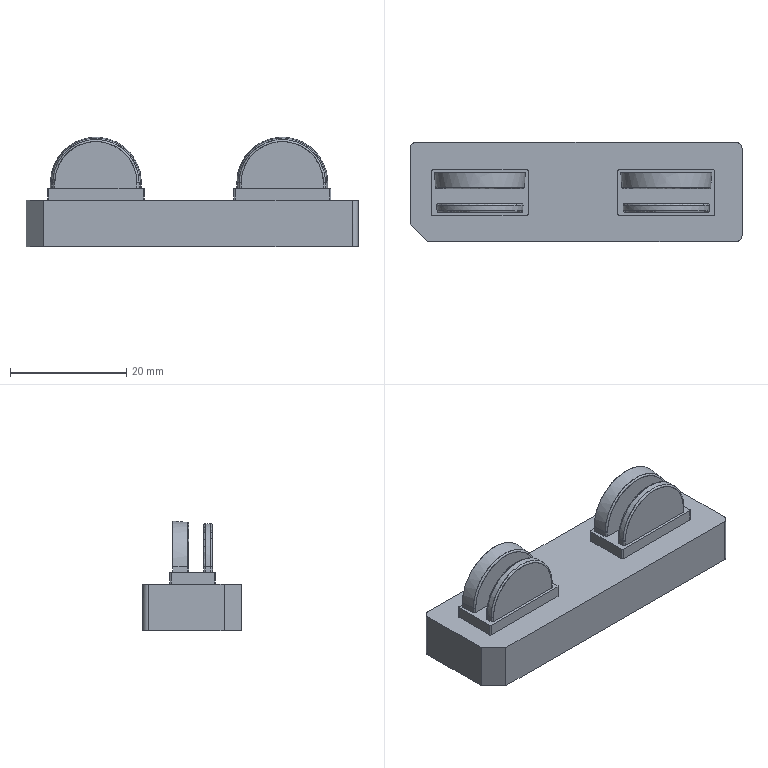NC program | PowerMill | posted by the shop | part box 57 x 17 x 18.807 mm
Lines 1 to 1576 of 381081:
%
G40 G49 G17 G80
( TOOL ID   D10C_1_1_1 )
( TOOL DIA. 10. TIP RAD 0 LENGTH 74.24 )
( Z = -.073 )
T1 M6
T2
G91 G28 Z0
G0 G90 G54
M08
S8000 M3
G0 X0 Y0 M8
G43 Z10.2 H1
X31.28 Y11.28
Z1.127
G1 Z-.073 F6000
X-31.28 F10000
Y5.64
X31.28
Y0
X-31.28
Y-5.64
X31.28
Y-11.28
X-31.28
X-36.28
G0 Z10.2
X-.5 Y-.118
Z9.877
X-21.098 Y16.843
Z.678
G1 Z-.522 F6000
Y16.316 F10000
G3 X-16.35 Y11.568 I4.747 J0
G1 X15.352
X15.355 Y8.566
X17.676 Y8.568
X18.449 Y8.526
X19.196 Y8.39
X19.996 Y8.118
X20.769 Y7.717
X21.543 Y7.115
X21.82 Y6.843
X22.316 Y6.216
X22.812 Y5.296
X23.065 Y4.523
X23.188 Y3.749
X23.2 Y2.976
X23.09 Y2.16
X22.231 Y-.891
X21.892 Y-1.665
X21.543 Y-2.219
X21.265 Y-2.567
X21.195 Y-2.686
X21.159 Y-2.819
X21.115 Y-3.188
X20.836 Y-3.928
X20.818 Y-3.986
X20.807 Y-4.046
X20.769 Y-4.365
X20.565 Y-4.759
X20.072 Y-5.449
X20.027 Y-5.526
X19.996 Y-5.611
X19.321 Y-6.305
X18.449 Y-6.916
X18.164 Y-7.079
X17.676 Y-7.342
X16.902 Y-7.626
X16.129 Y-7.78
X15.355 Y-7.816
X14.582 Y-7.737
X13.808 Y-7.536
X13.035 Y-7.197
X12.869 Y-7.079
X12.262 Y-6.727
X11.679 Y-6.305
X11.488 Y-6.14
X10.944 Y-5.532
X10.715 Y-5.24
X10.424 Y-4.759
X10.102 Y-3.985
X9.877 Y-3.142
X9.841 Y-2.83
X9.803 Y-2.688
X9.726 Y-2.563
X9.62 Y-2.438
X9.168 Y-1.773
X9.044 Y-1.502
X4.649 Y-3.853
G2 X2.985 Y-6.649 I-1.661 J-.904
G1 X-4.004 Y-6.64
G2 X-5.642 Y-4.028 I.002 J1.821
G1 X-5.409 Y-3.545
G3 X-4.361 Y-.594 I-13.071 J6.304
G1 X-4.022 Y.832
X-3.885 Y1.503
X-3.793 Y2.18
X-3.543 Y4.576
G2 X-1.556 Y6.369 I1.989 J-.207
G1 X.549 Y6.371
G2 X2.542 Y4.556 I.002 J-2.
G1 X2.79 Y1.901
G3 X3.83 Y-2.215 I13.718 J1.278
G1 X4.055 Y-2.743
X4.649 Y-3.853
X9.044 Y-1.502
X8.765 Y-.891
X8.105 Y1.429
X7.904 Y2.202
X7.799 Y2.976
X7.808 Y3.749
X7.935 Y4.523
X8.189 Y5.296
X8.394 Y5.73
X8.588 Y6.069
X9.182 Y6.843
X9.941 Y7.52
X10.715 Y7.986
X11.488 Y8.301
X12.262 Y8.485
X13.035 Y8.563
X15.355 Y8.566
X15.352 Y11.568
X30.585
G2 X31.585 Y10.568 I0 J-1.
G1 Y-10.804
G2 X30.585 Y-11.804 I-1. J0
G1 X26.011
Y-6.359
G2 X25.902 Y-6.25 I0 J.109
X26.121 Y-6.25 I.109 J0
X26.011 Y-6.359 I-.109 J0
G1 Y-11.804
X-31.585
G2 X-32.585 Y-10.804 I0 J1.
G1 Y-6.265
X-27.106
G2 X-26.915 Y-6.265 I.095 J0
X-27.106 Y-6.265 I-.095 J0
G1 X-32.585
Y10.568
G2 X-31.585 Y11.568 I1. J0
G1 X-16.35
X-16.355 Y8.564
X-14.035 Y8.561
X-13.262 Y8.485
X-12.488 Y8.301
X-11.715 Y7.984
X-10.941 Y7.52
X-10.185 Y6.843
X-9.592 Y6.069
X-9.394 Y5.73
X-9.192 Y5.296
X-8.935 Y4.523
X-8.812 Y3.749
X-8.801 Y2.976
X-8.906 Y2.202
X-9.102 Y1.429
X-9.765 Y-.891
X-10.108 Y-1.665
X-10.62 Y-2.438
X-10.723 Y-2.56
X-10.802 Y-2.688
X-10.84 Y-2.833
X-10.858 Y-3.01
X-11.085 Y-3.985
X-11.519 Y-4.759
X-11.715 Y-5.233
X-12.488 Y-6.145
X-13.262 Y-6.727
X-13.837 Y-7.079
X-14.035 Y-7.197
X-14.808 Y-7.536
X-15.582 Y-7.737
X-16.355 Y-7.816
X-17.129 Y-7.78
X-17.902 Y-7.626
X-18.676 Y-7.341
X-19.449 Y-6.916
X-20.322 Y-6.305
X-20.996 Y-5.615
X-21.582 Y-4.759
X-21.769 Y-4.365
X-21.915 Y-3.985
X-22.125 Y-3.131
X-22.159 Y-2.83
X-22.197 Y-2.688
X-22.275 Y-2.562
X-22.38 Y-2.438
X-22.543 Y-2.219
X-22.889 Y-1.665
X-23.235 Y-.891
X-23.439 Y-.118
X-24.09 Y2.16
X-24.203 Y2.976
X-24.19 Y3.749
X-24.09 Y4.411
X-23.81 Y5.296
X-23.41 Y6.069
X-22.819 Y6.843
X-22.543 Y7.115
X-21.924 Y7.616
X-20.996 Y8.117
X-20.222 Y8.383
X-19.449 Y8.526
X-18.676 Y8.568
X-16.355 Y8.564
X-16.35 Y11.568
G0 Z3.279
G1 X-21.098 Y16.843
G0 Z.279
G1 Z-.921 F6000
Y16.316 F10000
G3 X-16.35 Y11.568 I4.747 J0
G1 X-15.967
Y8.568
X-13.262
X-12.488 Y8.518
X-11.835 Y8.39
X-10.941 Y8.072
X-10.137 Y7.616
X-9.394 Y6.996
X-9.245 Y6.843
X-8.658 Y6.069
X-8.256 Y5.296
X-8.005 Y4.523
X-7.879 Y3.749
X-7.878 Y3.7
X-2.33 Y3.419
X-2.295 Y4.117
G2 X-.69 Y5.652 I1.605 J-.071
G1 X-.308 Y5.651
G2 X1.298 Y4.047 I0 J-1.606
G1 X1.3 Y2.368
G3 X2.006 Y-2.898 I20.231 J.03
G1 X2.177 Y-3.528
G2 X.239 Y-6.052 I-1.93 J-.524
G1 X-1.262 Y-6.046
G2 X-3.235 Y-3.768 I.008 J2.
G1 X-2.389 Y2.257
X-2.33 Y3.419
X-7.878 Y3.7
X-7.866 Y2.976
X-7.967 Y2.202
X-8.407 Y-.118
X-8.621 Y-.913
X-8.768 Y-1.29
X-8.878 Y-1.516
X-8.918 Y-1.635
X-8.928 Y-1.76
X-8.893 Y-2.438
X-8.964 Y-3.212
X-9.103 Y-3.985
X-9.277 Y-4.759
X-9.582 Y-5.532
X-10.048 Y-6.305
X-10.727 Y-7.079
X-10.941 Y-7.277
X-11.715 Y-7.842
X-12.488 Y-8.225
X-13.262 Y-8.496
X-13.825 Y-8.626
X-14.808 Y-8.754
X-15.582 Y-8.787
X-17.902 Y-8.774
X-18.676 Y-8.701
X-19.449 Y-8.569
X-20.222 Y-8.332
X-20.996 Y-8.003
X-21.268 Y-7.852
X-21.769 Y-7.516
X-22.278 Y-7.079
X-22.543 Y-6.799
X-22.952 Y-6.305
X-23.417 Y-5.532
X-23.723 Y-4.759
X-23.897 Y-3.985
X-24.034 Y-3.212
X-24.109 Y-2.438
X-24.072 Y-1.751
X-24.079 Y-1.635
X-24.113 Y-1.524
X-24.388 Y-.891
X-24.592 Y-.118
X-24.743 Y.655
X-25.032 Y2.202
X-25.131 Y2.976
X-25.123 Y3.749
X-24.993 Y4.523
X-24.742 Y5.296
X-24.343 Y6.069
X-24.09 Y6.436
X-23.751 Y6.843
X-23.316 Y7.264
X-22.86 Y7.616
X-22.543 Y7.819
X-21.769 Y8.194
X-21.165 Y8.39
X-20.222 Y8.549
X-19.449 Y8.568
X-18.676
X-18.672
X-15.967
Y11.568
X14.965
Y8.568
X17.669
X17.676
X18.449
X19.222 Y8.549
X19.996 Y8.431
X20.769 Y8.194
X21.543 Y7.819
X21.86 Y7.616
X22.316 Y7.264
X22.752 Y6.843
X23.09 Y6.436
X23.345 Y6.069
X23.742 Y5.296
X23.993 Y4.523
X24.124 Y3.749
X24.135 Y2.976
X24.033 Y2.202
X23.593 Y-.118
X23.387 Y-.891
X23.113 Y-1.524
X23.079 Y-1.635
X23.072 Y-1.751
X23.111 Y-2.438
X23.036 Y-3.212
X22.897 Y-3.985
X22.717 Y-4.759
X22.418 Y-5.532
X21.952 Y-6.305
X21.543 Y-6.799
X21.277 Y-7.079
X20.769 Y-7.516
X20.269 Y-7.852
X19.996 Y-8.003
X19.222 Y-8.332
X18.449 Y-8.569
X18.172 Y-8.626
X17.676 Y-8.701
X16.902 Y-8.774
X15.355 Y-8.797
X13.808 Y-8.754
X13.035 Y-8.661
X12.262 Y-8.496
X11.488 Y-8.225
X10.715 Y-7.842
X9.941 Y-7.277
X9.722 Y-7.079
X9.051 Y-6.305
X8.583 Y-5.532
X8.28 Y-4.759
X8.103 Y-3.985
X7.964 Y-3.212
X7.891 Y-2.438
X7.928 Y-1.761
X7.921 Y-1.647
X7.888 Y-1.537
X7.621 Y-.914
X7.41 Y-.118
X7.097 Y1.429
X6.866 Y2.976
X6.879 Y3.749
X7.007 Y4.523
X7.259 Y5.296
X7.621 Y6.012
X8.248 Y6.843
X8.394 Y6.996
X9.14 Y7.616
X9.941 Y8.072
X10.715 Y8.357
X11.488 Y8.518
X12.262 Y8.568
X14.965
Y11.568
X30.585
G2 X31.585 Y10.568 I0 J-1.
G1 Y-10.804
G2 X30.585 Y-11.804 I-1. J0
G1 X-31.585
G2 X-32.585 Y-10.804 I0 J1.
G1 Y10.568
G2 X-31.585 Y11.568 I1. J0
G1 X-16.35
G0 Z2.88
G1 X-21.098 Y16.843
G0 Z-.12
G1 Z-1.32 F6000
Y16.316 F10000
G3 X-16.35 Y11.568 I4.747 J0
G1 X15.355
Y8.568
X19.222
X19.996 Y8.547
X20.769 Y8.424
X21.543 Y8.178
X22.316 Y7.795
X22.595 Y7.616
X23.09 Y7.229
X23.484 Y6.843
X23.863 Y6.38
X24.073 Y6.069
X24.471 Y5.296
X24.722 Y4.523
X24.85 Y3.749
X24.861 Y2.976
X24.769 Y2.202
X24.413 Y-.118
X24.209 Y-.891
X24.039 Y-1.308
X24.006 Y-1.435
X24.007 Y-1.566
X24.021 Y-1.665
X24.062 Y-2.438
X23.896 Y-3.985
X23.723 Y-4.759
X23.419 Y-5.532
X22.958 Y-6.305
X22.311 Y-7.079
X21.543 Y-7.706
X20.769 Y-8.158
X19.996 Y-8.468
X19.394 Y-8.626
X18.449 Y-8.768
X17.676 Y-8.804
X13.035 Y-8.799
X12.262 Y-8.741
X11.606 Y-8.626
X10.715 Y-8.368
X9.941 Y-8.005
X9.168 Y-7.498
X8.688 Y-7.079
X8.394 Y-6.761
X8.042 Y-6.305
X7.621 Y-5.613
X7.277 Y-4.759
X7.104 Y-3.985
X6.939 Y-2.438
X6.979 Y-1.665
X6.993 Y-1.573
Y-1.437
X6.958 Y-1.307
X6.848 Y-1.046
X6.587 Y-.118
X6.351 Y1.429
X6.139 Y2.976
X6.147 Y3.557
X.627 Y3.902
X.615 Y3.704
G3 X1.332 Y-2.91 I19.557 J-1.225
G1 X1.509 Y-3.528
G2 X-.382 Y-5.994 I-1.86 J-.532
G1 X-.673 Y-5.989
G2 X-2.555 Y-3.77 I.031 J1.934
G1 X-1.638 Y2.447
X-1.613 Y3.417
X-1.664 Y4.502
G2 X-.833 Y5.381 I.831 J.047
G1 X-.167 Y5.382
G2 X.664 Y4.497 I0 J-.833
G1 X.627 Y3.902
X6.147 Y3.557
X6.15 Y3.749
X6.277 Y4.523
X6.529 Y5.296
X6.848 Y5.937
X7.516 Y6.843
X8.394 Y7.609
X9.168 Y8.055
X9.941 Y8.348
X10.715 Y8.514
X11.488 Y8.568
X15.355
Y11.568
X30.585
G2 X31.585 Y10.568 I0 J-1.
G1 Y-10.804
G2 X30.585 Y-11.804 I-1. J0
G1 X-31.585
G2 X-32.585 Y-10.804 I0 J1.
G1 Y10.568
G2 X-31.585 Y11.568 I1. J0
G1 X-16.355
Y8.568
X-12.488
X-11.715 Y8.514
X-11.094 Y8.39
X-10.168 Y8.055
X-9.405 Y7.616
X-8.621 Y6.953
X-7.927 Y6.069
X-7.529 Y5.296
X-7.277 Y4.523
X-7.15 Y3.749
X-7.139 Y2.976
X-7.231 Y2.202
X-7.587 Y-.118
X-7.793 Y-.891
X-7.962 Y-1.308
X-7.995 Y-1.435
X-7.993 Y-1.566
X-7.979 Y-1.665
X-7.938 Y-2.438
X-8.105 Y-3.985
X-8.277 Y-4.759
X-8.581 Y-5.532
X-9.042 Y-6.305
X-9.394 Y-6.761
X-9.688 Y-7.079
X-10.168 Y-7.498
X-10.941 Y-8.005
X-11.715 Y-8.368
X-12.607 Y-8.626
X-13.262 Y-8.741
X-14.035 Y-8.799
X-18.676 Y-8.804
X-19.449 Y-8.768
X-20.222 Y-8.662
X-20.996 Y-8.468
X-21.769 Y-8.158
X-22.543 Y-7.706
X-23.316 Y-7.072
X-23.957 Y-6.305
X-24.09 Y-6.113
X-24.417 Y-5.532
X-24.723 Y-4.759
X-24.863 Y-4.179
X-25.061 Y-2.438
X-25.021 Y-1.665
X-25.007 Y-1.569
X-25.006 Y-1.437
X-25.039 Y-1.309
X-25.21 Y-.891
X-25.413 Y-.118
X-25.636 Y1.353
X-25.861 Y2.976
X-25.85 Y3.749
X-25.723 Y4.523
X-25.471 Y5.296
X-25.073 Y6.069
X-24.863 Y6.38
X-24.484 Y6.843
X-24.09 Y7.229
X-23.595 Y7.616
X-23.316 Y7.795
X-22.543 Y8.178
X-21.906 Y8.39
X-20.996 Y8.547
X-20.222 Y8.568
X-16.355
Y11.568
X-16.35
G0 Z2.481
G1 X-21.098 Y16.843
G0 Z-.519
G1 Z-1.719 F6000
Y16.316 F10000
G3 X-16.35 Y11.568 I4.747 J0
G1 X15.742
Y8.568
X19.996
X20.769 Y8.527
X21.486 Y8.39
X22.316 Y8.095
X23.09 Y7.669
X23.863 Y7.041
X24.057 Y6.843
X24.646 Y6.069
X25.043 Y5.296
X25.296 Y4.523
X25.41 Y3.865
X25.434 Y2.976
X25.043 Y-.118
X24.84 Y-.891
X24.722 Y-1.191
X24.689 Y-1.324
X24.694 Y-1.46
X24.696 Y-1.472
X24.763 Y-2.438
X24.636 Y-3.823
X24.441 Y-4.759
X24.139 Y-5.532
X23.693 Y-6.305
X23.09 Y-7.036
X22.316 Y-7.685
X22.073 Y-7.852
X21.543 Y-8.153
X20.769 Y-8.466
X20.234 Y-8.626
X19.996 Y-8.678
X19.222 Y-8.778
X18.449 Y-8.804
X12.262
X11.488 Y-8.751
X10.766 Y-8.626
X9.941 Y-8.365
X9.168 Y-7.999
X8.927 Y-7.852
X8.394 Y-7.47
X7.952 Y-7.079
X7.621 Y-6.719
X7.307 Y-6.305
X6.848 Y-5.506
X6.556 Y-4.759
X6.385 Y-3.985
X6.237 Y-2.438
X6.277 Y-1.665
X6.31 Y-1.451
X6.314 Y-1.325
X6.286 Y-1.202
X6.074 Y-.62
X5.959 Y-.118
X5.566 Y2.976
X5.577 Y3.749
X5.704 Y4.523
X5.957 Y5.296
X6.355 Y6.069
X6.848 Y6.734
X7.621 Y7.461
X7.832 Y7.616
X8.394 Y7.955
X9.168 Y8.285
X9.515 Y8.39
X9.941 Y8.482
X10.715 Y8.564
X11.488 Y8.568
X15.742
Y11.568
X30.585
G2 X31.585 Y10.568 I0 J-1.
G1 Y-10.804
G2 X30.585 Y-11.804 I-1. J0
G1 X-31.585
G2 X-32.585 Y-10.804 I0 J1.
G1 Y10.568
G2 X-31.585 Y11.568 I1. J0
G1 X-17.129
Y8.568
X-13.262
X-13.243
X-12.488
X-12.46 Y8.566
X-11.715 Y8.564
X-10.941 Y8.482
X-10.514 Y8.39
X-10.168 Y8.285
X-9.394 Y7.955
X-8.832 Y7.616
X-8.621 Y7.461
X-7.943 Y6.843
X-7.355 Y6.069
X-7.074 Y5.558
X-6.956 Y5.296
X-6.704 Y4.523
X-6.577 Y3.749
X-6.567 Y2.976
X-6.952 Y-.076
X-1.037 Y-.895
X-.884 Y.208
X-.789 Y.956
X-.709 Y1.706
X-.662 Y2.2
G3 X-.628 Y3.905 I-11.295 J1.077
G1 X-.633 Y4.
X-.679 Y4.525
X-.758 Y5.046
X-.799 Y5.271
G2 X-.509 Y5.62 I.291 J.053
G1 X-.491
G2 X-.201 Y5.269 I0 J-.296
G1 X-.227 Y5.133
X-.318 Y4.55
X-.369 Y3.961
X-.374 Y3.855
G3 X-.321 Y2.032 I11.214 J-.584
G1 X-.203 Y.969
X-.157 Y.571
X-.105 Y.173
X.185 Y-1.968
X.362 Y-3.754
X.395 Y-4.054
X.433 Y-4.354
X.493 Y-4.794
X.529 Y-5.022
X.573 Y-5.247
X.632 Y-5.517
G2 X.359 Y-5.856 I-.273 J-.059
G1 X-1.36
G2 X-1.632 Y-5.514 I0 J.279
G1 X-1.604 Y-5.393
X-1.546 Y-5.117
X-1.499 Y-4.839
X-1.451 Y-4.514
X-1.4 Y-4.133
X-1.359 Y-3.751
X-1.19 Y-1.998
X-1.037 Y-.895
X-6.952 Y-.076
X-6.957 Y-.118
X-7.074 Y-.62
X-7.284 Y-1.197
X-7.313 Y-1.324
X-7.307 Y-1.453
X-7.304 Y-1.472
X-7.237 Y-2.438
X-7.385 Y-3.985
X-7.557 Y-4.759
X-7.848 Y-5.506
X-8.307 Y-6.305
X-8.621 Y-6.719
X-8.952 Y-7.079
X-9.394 Y-7.47
X-9.927 Y-7.852
X-10.168 Y-7.999
X-10.941 Y-8.365
X-11.766 Y-8.626
X-12.488 Y-8.751
X-13.262 Y-8.804
X-19.449
X-20.222 Y-8.778
X-20.996 Y-8.678
X-21.769 Y-8.466
X-22.543 Y-8.153
X-23.073 Y-7.852
X-23.316 Y-7.685
X-24.048 Y-7.079
X-24.693 Y-6.305
X-25.14 Y-5.532
X-25.442 Y-4.759
X-25.616 Y-3.985
X-25.763 Y-2.438
X-25.723 Y-1.665
X-25.69 Y-1.457
X-25.687 Y-1.326
X-25.719 Y-1.198
X-25.839 Y-.891
X-26.042 Y-.118
X-26.434 Y2.976
X-26.423 Y3.749
X-26.296 Y4.523
X-26.044 Y5.296
X-25.636 Y6.081
X-25.057 Y6.843
X-24.863 Y7.041
X-24.168 Y7.616
X-23.316 Y8.095
X-22.543 Y8.373
X-21.769 Y8.527
X-20.996 Y8.568
X-17.129
Y11.568
X-16.35
G0 Z2.082
G1 X-21.098 Y16.843
G0 Z-.918
G1 Z-2.118 F6000
Y16.316 F10000
G3 X-16.35 Y11.568 I4.747 J0
G1 X-.5
Y5.891
G2 X-.346 Y5.737 I0 J-.154
X-.654 Y5.737 I-.154 J0
X-.5 Y5.891 I.154 J0
G1 Y11.568
X15.742
Y8.568
X19.996
X20.046 Y8.565
X20.769
X21.543 Y8.485
X21.98 Y8.39
X22.316 Y8.289
X23.09 Y7.959
X23.657 Y7.616
X23.863 Y7.465
X24.543 Y6.843
X25.131 Y6.069
X25.528 Y5.296
X25.78 Y4.523
X25.907 Y3.749
X25.918 Y2.976
X25.563 Y-.118
X25.41 Y-.739
X25.262 Y-1.139
X25.233 Y-1.263
X25.237 Y-1.39
X25.28 Y-1.665
X25.321 Y-2.438
X25.183 Y-3.985
X25.011 Y-4.759
X24.709 Y-5.532
X24.274 Y-6.305
X23.863 Y-6.831
X23.631 Y-7.079
X23.09 Y-7.552
X22.675 Y-7.852
X22.316 Y-8.065
X21.543 Y-8.412
X20.867 Y-8.626
X19.996 Y-8.768
X19.222 Y-8.804
X18.454
X18.449
X12.262
X12.234 Y-8.802
X11.488
X10.715 Y-8.735
X10.133 Y-8.626
X9.168 Y-8.298
X8.394 Y-7.896
X7.621 Y-7.313
X7.369 Y-7.079
X6.848 Y-6.475
X6.727 Y-6.305
X6.289 Y-5.532
X5.992 Y-4.759
X5.818 Y-3.985
X5.729 Y-2.993
X.341 Y-3.496
X.493 Y-5.126
G2 X-.339 Y-6.02 I-.814 J-.076
G1 X-.678 Y-6.012
G2 X-1.481 Y-5.096 I.018 J.826
G1 X-1.269 Y-3.108
X-1.191 Y-1.891
G2 X.189 Y-1.866 I.691 J-.04
G1 X.341 Y-3.496
X5.729 Y-2.993
X5.679 Y-2.438
X5.718 Y-1.665
X5.761 Y-1.402
X5.764 Y-1.265
X5.731 Y-1.132
X5.707 Y-1.075
X5.439 Y-.118
X5.082 Y2.976
X5.093 Y3.749
X5.22 Y4.523
X5.472 Y5.296
X5.869 Y6.069
X6.074 Y6.371
X6.457 Y6.843
X6.848 Y7.226
X7.343 Y7.616
X7.621 Y7.796
X8.394 Y8.182
X9.02 Y8.39
X9.941 Y8.549
X10.715 Y8.568
X11.452
X11.488
X15.742
Y11.568
X30.585
G2 X31.585 Y10.568 I0 J-1.
G1 Y-10.804
G2 X30.585 Y-11.804 I-1. J0
G1 X-31.585
G2 X-32.585 Y-10.804 I0 J1.
G1 Y10.568
G2 X-31.585 Y11.568 I1. J0
G1 X-17.129
Y8.568
X-13.262
X-13.243
X-12.488
X-12.486
X-11.715
X-10.941 Y8.549
X-10.168 Y8.426
X-9.394 Y8.182
X-8.621 Y7.796
X-8.343 Y7.616
X-7.848 Y7.226
X-7.457 Y6.843
X-7.074 Y6.372
X-6.869 Y6.069
X-6.472 Y5.296
X-6.22 Y4.523
X-6.093 Y3.749
X-6.082 Y2.976
X-6.437 Y-.118
X-6.64 Y-.891
X-6.735 Y-1.136
X-6.766 Y-1.263
X-6.762 Y-1.394
X-6.72 Y-1.665
X-6.678 Y-2.438
X-6.82 Y-3.985
X-6.992 Y-4.759
X-7.291 Y-5.532
X-7.726 Y-6.305
X-8.369 Y-7.079
X-8.621 Y-7.313
X-9.325 Y-7.852
X-10.168 Y-8.298
X-11.133 Y-8.626
X-11.715 Y-8.735
X-12.488 Y-8.802
X-13.234
X-13.262 Y-8.804
X-19.449
X-19.454
X-20.222
X-20.996 Y-8.768
X-21.769 Y-8.648
X-22.543 Y-8.412
X-23.316 Y-8.065
X-23.675 Y-7.852
X-24.09 Y-7.552
X-24.631 Y-7.079
X-24.863 Y-6.831
X-25.274 Y-6.305
X-25.636 Y-5.687
X-26.01 Y-4.759
X-26.18 Y-3.985
X-26.322 Y-2.438
X-26.282 Y-1.665
X-26.237 Y-1.392
X-26.233 Y-1.264
X-26.262 Y-1.139
X-26.41 Y-.735
X-26.56 Y-.118
X-26.918 Y2.976
X-26.907 Y3.749
X-26.78 Y4.523
X-26.528 Y5.296
X-26.131 Y6.069
X-25.636 Y6.736
X-24.863 Y7.466
X-24.657 Y7.616
X-24.09 Y7.959
X-23.316 Y8.289
X-22.98 Y8.39
X-22.543 Y8.485
X-21.769 Y8.565
X-21.046
X-20.996 Y8.568
X-17.129
Y11.568
X-16.35
G0 Z1.683
G1 X-21.098 Y16.843
G0 Z-1.317
G1 Z-2.517 F6000
Y16.316 F10000
G3 X-16.35 Y11.568 I4.747 J0
G1 X15.355
Y8.568
X20.769
X21.543 Y8.543
X22.316 Y8.414
X23.09 Y8.161
X23.863 Y7.762
X24.086 Y7.616
X24.636 Y7.176
X24.97 Y6.843
X25.41 Y6.291
X25.557 Y6.069
X25.954 Y5.296
X26.183 Y4.607
X26.332 Y3.749
X26.343 Y2.976
X26. Y-.118
X25.797 Y-.891
X25.72 Y-1.092
X25.69 Y-1.221
X25.694 Y-1.354
X25.747 Y-1.665
X25.785 Y-2.438
X25.657 Y-3.985
X25.484 Y-4.759
X25.19 Y-5.532
X24.754 Y-6.305
X24.636 Y-6.472
X24.113 Y-7.079
X23.863 Y-7.312
X23.17 Y-7.852
X22.316 Y-8.303
X21.384 Y-8.626
X20.769 Y-8.74
X19.996 Y-8.804
X19.229
X19.222
X18.454
X18.449
X15.719
X11.488
X10.715 Y-8.791
X9.941 Y-8.695
X9.615 Y-8.626
X9.168 Y-8.494
X8.394 Y-8.172
X7.83 Y-7.852
X7.621 Y-7.709
X6.887 Y-7.079
X6.245 Y-6.305
X6.074 Y-6.034
X5.809 Y-5.532
X5.515 Y-4.759
X5.344 Y-3.985
X5.214 Y-2.438
X5.253 Y-1.665
X5.306 Y-1.357
X5.31 Y-1.225
X5.281 Y-1.097
X5.203 Y-.891
X5.001 Y-.118
X4.657 Y2.976
X4.668 Y3.749
X4.795 Y4.523
X-.492 Y6.039
X-.496 Y6.025
X-.5 Y6.01
X-.508 Y6.039
X-.517 Y6.068
X-.484
X-.488 Y6.054
X-.492 Y6.039
X4.795 Y4.523
X5.046 Y5.296
X5.443 Y6.069
X6.03 Y6.843
X6.848 Y7.568
X7.621 Y8.03
X8.394 Y8.334
X9.168 Y8.509
X9.941 Y8.568
X15.355
Y11.568
X30.585
G2 X31.585 Y10.568 I0 J-1.
G1 Y-10.804
G2 X30.585 Y-11.804 I-1. J0
G1 X-31.585
G2 X-32.585 Y-10.804 I0 J1.
G1 Y10.568
G2 X-31.585 Y11.568 I1. J0
G1 X-16.355
Y8.568
X-10.941
X-10.168 Y8.509
X-9.394 Y8.334
X-8.621 Y8.03
X-7.914 Y7.616
X-7.074 Y6.89
X-6.443 Y6.069
X-6.046 Y5.296
X-5.795 Y4.523
X-5.668 Y3.749
X-5.657 Y2.976
X-6. Y-.118
X-6.203 Y-.891
X-6.28 Y-1.093
X-6.311 Y-1.222
X-6.306 Y-1.355
X-6.253 Y-1.665
X-6.214 Y-2.438
X-6.266 Y-3.069
X-.916 Y-3.401
X-.892 Y-2.811
X-.893 Y-2.22
X-.901 Y-1.91
G2 X-.498 Y-1.499 I.401 J.01
X-.099 Y-1.914 I-.002 J-.401
G1 X-.116 Y-2.525
X.058 Y-4.652
X.088 Y-4.866
X.226 Y-5.574
G2 X-.66 Y-6.377 I-.686 J-.133
G1 X-.708 Y-6.363
G2 X-1.193 Y-5.601 I.196 J.66
G1 X-1.04 Y-4.576
X-.965 Y-3.99
X-.916 Y-3.401
X-6.266 Y-3.069
X-6.343 Y-3.985
X-6.515 Y-4.759
X-6.81 Y-5.532
X-7.074 Y-6.034
X-7.246 Y-6.305
X-7.848 Y-7.037
X-8.621 Y-7.709
X-8.83 Y-7.852
X-9.394 Y-8.172
X-10.168 Y-8.494
X-10.615 Y-8.626
X-10.941 Y-8.695
X-11.715 Y-8.791
X-12.488 Y-8.804
X-16.719
X-19.449
X-19.454
X-20.222
X-20.229
X-20.996
X-21.769 Y-8.74
X-22.385 Y-8.626
X-23.316 Y-8.303
X-24.09 Y-7.904
X-24.863 Y-7.312
X-25.112 Y-7.079
X-25.636 Y-6.472
X-25.755 Y-6.305
X-26.191 Y-5.532
X-26.484 Y-4.759
X-26.657 Y-3.985
X-26.786 Y-2.438
X-26.747 Y-1.665
X-26.695 Y-1.357
X-26.69 Y-1.226
X-26.719 Y-1.098
X-26.797 Y-.891
X-26.999 Y-.118
X-27.343 Y2.976
X-27.332 Y3.749
X-27.205 Y4.523
X-26.954 Y5.296
X-26.557 Y6.069
X-26.41 Y6.29
X-25.97 Y6.843
X-25.636 Y7.176
X-25.086 Y7.616
X-24.863 Y7.763
X-24.09 Y8.161
X-23.413 Y8.39
X-22.543 Y8.543
X-21.769 Y8.568
X-16.355
Y11.568
X-16.35
G0 Z1.284
G1 X-21.098 Y16.843
G0 Z-1.716
G1 Z-2.916 F6000
Y16.316 F10000
G3 X-16.35 Y11.568 I4.747 J0
G1 X15.503
Y8.568
X20.769
X20.834 Y8.566
X21.543
X22.316 Y8.488
X22.772 Y8.39
X23.09 Y8.293
X23.863 Y7.968
X24.445 Y7.616
X24.636 Y7.477
X25.33 Y6.843
X25.916 Y6.069
X26.183 Y5.583
X26.313 Y5.296
X26.565 Y4.523
X26.691 Y3.749
X26.702 Y2.976
X26.381 Y-.118
X26.178 Y-.891
X26.115 Y-1.059
X26.085 Y-1.188
X26.09 Y-1.32
X26.149 Y-1.665
X26.189 Y-2.438
X26.067 Y-3.985
X25.895 Y-4.759
X25.598 Y-5.532
X25.41 Y-5.903
X25.163 Y-6.305
X24.636 Y-6.96
X23.863 Y-7.66
X23.589 Y-7.852
X23.09 Y-8.14
X22.316 Y-8.476
X21.821 Y-8.626
X21.543 Y-8.686
X20.769 Y-8.789
X19.996 Y-8.804
X10.715
X9.941 Y-8.76
X9.178 Y-8.626
X8.394 Y-8.365
X7.621 Y-7.982
X7.41 Y-7.852
X6.848 Y-7.428
X6.479 Y-7.079
X6.074 Y-6.625
X5.837 Y-6.305
X5.403 Y-5.532
X5.104 Y-4.759
X4.933 Y-3.985
X4.811 Y-2.438
X4.851 Y-1.665
X4.91 Y-1.321
X4.915 Y-1.19
X4.886 Y-1.061
X4.822 Y-.891
X4.619 Y-.118
X4.298 Y2.976
X4.309 Y3.749
X4.433 Y4.511
X-.007 Y5.239
X4.433 Y4.511
X4.435 Y4.523
X4.687 Y5.296
X5.084 Y6.069
X5.301 Y6.391
X5.67 Y6.843
X6.074 Y7.238
X6.555 Y7.616
X6.848 Y7.805
X7.621 Y8.189
X8.227 Y8.39
X9.168 Y8.55
X9.941 Y8.568
X10.236
X15.503
Y11.568
X30.585
G2 X31.585 Y10.568 I0 J-1.
G1 Y-10.804
G2 X30.585 Y-11.804 I-1. J0
G1 X-.5
Y-7.304
X-1.534
G2 X-2.001 Y-6.625 I0 J.5
G1 X-1.904 Y-6.371
X-1.797 Y-6.057
X-1.713 Y-5.737
X-1.54 Y-4.963
X-1.483 Y-4.653
X-1.447 Y-4.339
X-1.325 Y-2.792
X-1.311 Y-2.499
X-1.317 Y-2.206
X-1.345 Y-1.654
X-1.343 Y-1.578
X-1.33 Y-1.502
X-1.265 Y-1.257
X-1.191 Y-.922
X-1.143 Y-.583
X-.997 Y.821
G2 X-.003 Y.821 I.497 J-.052
G1 X.143 Y-.583
X.192 Y-.924
X.266 Y-1.259
X.33 Y-1.5
X.343 Y-1.576
X.345 Y-1.653
X.317 Y-2.208
X.311 Y-2.5
X.325 Y-2.792
X.447 Y-4.339
X.482 Y-4.65
X.539 Y-4.958
X.711 Y-5.732
X.796 Y-6.059
X.906 Y-6.379
X1.001 Y-6.624
G2 X.534 Y-7.304 I-.466 J-.18
G1 X-.5
Y-11.804
X-31.585
G2 X-32.585 Y-10.804 I0 J1.
G1 Y10.568
G2 X-31.585 Y11.568 I1. J0
G1 X-16.503
Y8.568
X-11.236
X-10.941
X-10.168 Y8.55
X-9.394 Y8.431
X-8.621 Y8.189
X-7.848 Y7.805
X-7.555 Y7.616
X-7.074 Y7.239
X-6.67 Y6.843
X-6.301 Y6.389
X-6.084 Y6.069
X-5.687 Y5.296
X-5.527 Y4.853
X-5.437 Y4.523
X-5.309 Y3.749
X-5.298 Y2.976
X-5.619 Y-.118
X-5.821 Y-.891
X-5.885 Y-1.059
X-5.915 Y-1.188
X-5.91 Y-1.32
X-5.851 Y-1.665
X-5.811 Y-2.438
X-5.933 Y-3.985
X-6.105 Y-4.759
X-6.402 Y-5.532
X-6.837 Y-6.305
X-7.074 Y-6.625
X-7.478 Y-7.079
X-7.848 Y-7.428
X-8.41 Y-7.852
X-8.621 Y-7.982
X-9.394 Y-8.365
X-10.178 Y-8.626
X-10.941 Y-8.76
X-11.715 Y-8.804
X-20.996
X-21.769 Y-8.789
X-22.543 Y-8.686
X-23.316 Y-8.476
X-24.09 Y-8.14
X-24.589 Y-7.852
X-24.863 Y-7.66
X-25.521 Y-7.079
X-26.162 Y-6.305
X-26.41 Y-5.903
X-26.598 Y-5.532
X-26.895 Y-4.759
X-27.067 Y-3.985
X-27.189 Y-2.438
X-27.149 Y-1.665
X-27.09 Y-1.321
X-27.085 Y-1.189
X-27.115 Y-1.06
X-27.183 Y-.877
X-27.379 Y-.118
X-27.702 Y2.976
X-27.691 Y3.749
X-27.565 Y4.523
X-27.313 Y5.296
X-27.183 Y5.583
X-26.916 Y6.069
X-26.41 Y6.753
X-25.636 Y7.477
X-25.445 Y7.616
X-24.863 Y7.967
X-24.09 Y8.293
X-23.773 Y8.39
X-23.316 Y8.488
X-22.543 Y8.566
X-21.834
X-21.769 Y8.568
X-16.503
Y11.568
X-16.35
G0 Z.885
G1 X-21.098 Y16.843
G0 Z-2.115
G1 Z-3.315 F6000
Y16.316 F10000
G3 X-16.35 Y11.568 I4.747 J0
G1 X15.503
Y8.568
X20.769
X20.771
X21.543
X22.316 Y8.535
X23.093 Y8.39
X23.863 Y8.119
X24.636 Y7.7
X25.41 Y7.083
X25.644 Y6.843
X26.183 Y6.143
X26.627 Y5.296
X26.878 Y4.523
X27.005 Y3.749
X27.016 Y2.976
X26.705 Y-.118
X26.504 Y-.891
X26.45 Y-1.037
X26.421 Y-1.165
X26.426 Y-1.296
X26.49 Y-1.665
X26.53 Y-2.438
X26.409 Y-3.985
X26.237 Y-4.759
X25.951 Y-5.532
X25.516 Y-6.305
X24.882 Y-7.079
X24.636 Y-7.319
X23.952 Y-7.852
X23.09 Y-8.318
X22.197 Y-8.626
X21.543 Y-8.747
X20.769 Y-8.804
X10.715
X9.941 Y-8.795
X9.168 Y-8.703
X8.394 Y-8.507
X7.621 Y-8.179
X7.048 Y-7.852
X6.848 Y-7.714
X6.118 Y-7.079
X5.484 Y-6.305
X5.301 Y-6.016
X5.049 Y-5.532
X4.761 Y-4.759
X4.591 Y-3.985
X4.469 Y-2.438
X4.49 Y-2.026
X-.004 Y-1.796
X4.49 Y-2.026
X4.509 Y-1.665
X4.573 Y-1.296
X4.579 Y-1.166
X4.55 Y-1.038
X4.497 Y-.891
X4.295 Y-.118
X4.202 Y.655
X3.985 Y2.976
X3.995 Y3.749
X4.122 Y4.523
X4.255 Y4.932
X-.025 Y6.323
X4.255 Y4.932
X4.373 Y5.296
X4.527 Y5.634
X4.769 Y6.069
X5.301 Y6.781
X6.074 Y7.496
X6.848 Y7.982
X7.621 Y8.304
X8.394 Y8.494
X9.168 Y8.566
X9.885 Y8.567
X9.941 Y8.568
X10.236
X15.503
Y11.568
X30.585
G2 X31.585 Y10.568 I0 J-1.
G1 Y-10.804
G2 X30.585 Y-11.804 I-1. J0
G1 X-31.585
G2 X-32.585 Y-10.804 I0 J1.
G1 Y10.568
G2 X-31.585 Y11.568 I1. J0
G1 X-16.503
Y8.568
X-11.236
X-10.941
X-10.885 Y8.567
X-10.168 Y8.566
X-9.394 Y8.494
X-8.621 Y8.304
X-7.848 Y7.982
X-7.074 Y7.496
X-6.355 Y6.843
X-5.769 Y6.069
X-5.527 Y5.634
X-5.373 Y5.296
X-5.122 Y4.523
X-4.996 Y3.749
X-4.984 Y2.976
X-5.202 Y.655
X-5.295 Y-.118
X-5.497 Y-.891
X-5.55 Y-1.035
X-5.578 Y-1.164
X-5.572 Y-1.297
X-5.527 Y-1.547
X-5.471 Y-2.438
X-5.486 Y-2.636
X-.999 Y-2.98
X-5.486 Y-2.636
X-5.59 Y-3.985
X-5.761 Y-4.759
X-6.049 Y-5.532
X-6.301 Y-6.016
X-6.484 Y-6.305
X-7.074 Y-7.032
X-7.848 Y-7.714
X-8.048 Y-7.852
X-8.621 Y-8.179
X-9.394 Y-8.507
X-9.803 Y-8.626
X-10.168 Y-8.703
X-10.941 Y-8.795
X-11.715 Y-8.804
X-21.769
X-22.543 Y-8.747
X-23.197 Y-8.626
X-24.09 Y-8.318
X-24.863 Y-7.908
X-25.636 Y-7.319
X-25.882 Y-7.079
X-26.516 Y-6.305
X-26.951 Y-5.532
X-27.183 Y-4.928
X-27.411 Y-3.985
X-27.531 Y-2.438
X-27.491 Y-1.665
X-27.427 Y-1.297
X-27.421 Y-1.166
X-27.449 Y-1.039
X-27.503 Y-.891
X-27.705 Y-.118
X-28.016 Y2.976
X-28.004 Y3.749
X-27.878 Y4.523
X-27.627 Y5.296
X-27.23 Y6.069
X-26.644 Y6.843
X-26.41 Y7.083
X-25.762 Y7.616
X-24.863 Y8.119
X-24.09 Y8.39
X-23.316 Y8.535
X-22.543 Y8.568
X-21.771
X-21.769
X-16.503
Y11.568
X-16.35
G0 Z.486
G1 X-21.098 Y16.843
G0 Z-2.514
G1 Z-3.714 F6000
Y16.316 F10000
G3 X-16.35 Y11.568 I4.747 J0
G1 X15.355
Y8.568
X21.543
X22.316 Y8.559
X23.09 Y8.457
X23.863 Y8.237
X24.636 Y7.876
X25.049 Y7.616
X25.41 Y7.342
X25.933 Y6.843
X26.183 Y6.548
X26.517 Y6.069
X26.915 Y5.296
X27.166 Y4.523
X27.291 Y3.749
X27.302 Y2.976
X27.077 Y.655
X26.957 Y-.307
X26.738 Y-1.032
X26.718 Y-1.143
X26.723 Y-1.256
X26.79 Y-1.665
X26.829 Y-2.438
X26.716 Y-3.985
X26.544 Y-4.759
X26.262 Y-5.532
X25.827 Y-6.305
X25.41 Y-6.844
X25.197 Y-7.079
X24.636 Y-7.588
X24.27 Y-7.852
X23.863 Y-8.093
X23.09 Y-8.448
X22.515 Y-8.626
X21.543 Y-8.785
X20.769 Y-8.804
X9.941
X9.168 Y-8.752
X8.485 Y-8.626
X7.621 Y-8.33
X6.848 Y-7.927
X6.074 Y-7.343
X5.802 Y-7.079
X5.173 Y-6.305
X4.738 Y-5.532
X4.456 Y-4.759
X4.284 Y-3.985
X4.171 Y-2.438
X4.211 Y-1.665
X4.275 Y-1.27
X4.28 Y-1.146
X4.254 Y-1.025
X4.207 Y-.891
X4.006 Y-.118
X3.697 Y2.976